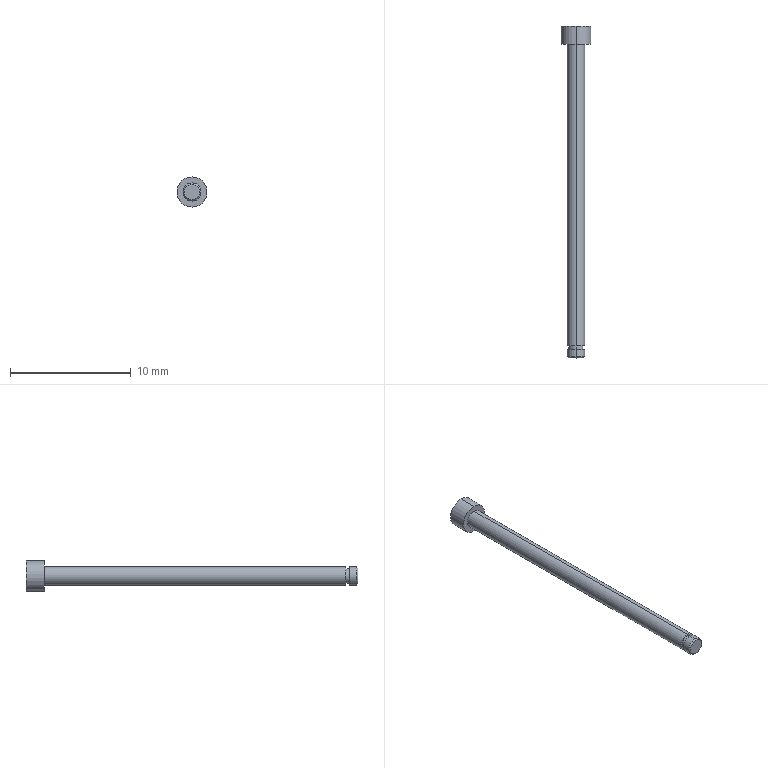Part | SolidWorks | features ICE 2, Chamfer 1, Extrusion 1 | 1 solid | 15 faces | box 2.5 x 27.5 x 2.5 mm | volume 53.096 mm3 | cylinder 8 | plane 5 | cone 2 | commonest cylinder face diameters 1.5 x4 1.2 x2 2.5 x2
STEP:
#1=CARTESIAN_POINT('',(0.,0.,-0.65));
#2=VERTEX_POINT('',#1);
#3=CARTESIAN_POINT('',(0.,0.,0.65));
#4=VERTEX_POINT('',#3);
#5=CARTESIAN_POINT('',(0.,0.,0.));
#6=DIRECTION('',(0.,-1.,0.));
#7=DIRECTION('',(0.,0.,1.));
#8=AXIS2_PLACEMENT_3D('',#5,#6,#7);
#9=CIRCLE('',#8,0.65);
#10=EDGE_CURVE('',#2,#4,#9,.T.);
#11=ORIENTED_EDGE('',*,*,#10,.F.);
#12=CARTESIAN_POINT('',(0.,0.1,-0.75));
#13=VERTEX_POINT('',#12);
#14=CARTESIAN_POINT('',(0.,0.1,-0.75));
#15=DIRECTION('',(0.,0.7071,-0.7071));
#16=VECTOR('',#15,1000.);
#17=LINE('',#14,#16);
#18=EDGE_CURVE('',#2,#13,#17,.T.);
#19=ORIENTED_EDGE('',*,*,#18,.T.);
#20=CARTESIAN_POINT('',(0.,0.1,0.75));
#21=VERTEX_POINT('',#20);
#22=CARTESIAN_POINT('',(0.,0.1,0.));
#23=DIRECTION('',(0.,1.,0.));
#24=DIRECTION('',(0.,0.,1.));
#25=AXIS2_PLACEMENT_3D('',#22,#23,#24);
#26=CIRCLE('',#25,0.75);
#27=EDGE_CURVE('',#21,#13,#26,.T.);
#28=ORIENTED_EDGE('',*,*,#27,.F.);
#29=CARTESIAN_POINT('',(0.,0.1,0.75));
#30=DIRECTION('',(0.,0.7071,0.7071));
#31=VECTOR('',#30,1000.);
#32=LINE('',#29,#31);
#33=EDGE_CURVE('',#4,#21,#32,.T.);
#34=ORIENTED_EDGE('',*,*,#33,.F.);
#35=EDGE_LOOP('',(#11,#19,#28,#34));
#36=FACE_OUTER_BOUND('',#35,.T.);
#37=CARTESIAN_POINT('',(0.,0.1,0.));
#38=DIRECTION('',(0.,1.,0.));
#39=DIRECTION('',(0.,0.,1.));
#40=AXIS2_PLACEMENT_3D('',#37,#38,#39);
#41=CONICAL_SURFACE('',#40,0.75,0.7854);
#42=ADVANCED_FACE('',(#36),#41,.T.);
#43=CARTESIAN_POINT('',(0.,0.7,-0.75));
#44=VERTEX_POINT('',#43);
#45=CARTESIAN_POINT('',(0.,0.7,0.75));
#46=VERTEX_POINT('',#45);
#47=CARTESIAN_POINT('',(0.,0.7,0.));
#48=DIRECTION('',(0.,-1.,0.));
#49=DIRECTION('',(0.,0.,-1.));
#50=AXIS2_PLACEMENT_3D('',#47,#48,#49);
#51=CIRCLE('',#50,0.75);
#52=EDGE_CURVE('',#44,#46,#51,.T.);
#53=ORIENTED_EDGE('',*,*,#52,.T.);
#54=CARTESIAN_POINT('',(0.,26.,0.75));
#55=DIRECTION('',(0.,-1.,0.));
#56=VECTOR('',#55,1000.);
#57=LINE('',#54,#56);
#58=EDGE_CURVE('',#46,#21,#57,.T.);
#59=ORIENTED_EDGE('',*,*,#58,.T.);
#60=ORIENTED_EDGE('',*,*,#27,.T.);
#61=CARTESIAN_POINT('',(0.,26.,-0.75));
#62=DIRECTION('',(0.,-1.,0.));
#63=VECTOR('',#62,1000.);
#64=LINE('',#61,#63);
#65=EDGE_CURVE('',#44,#13,#64,.T.);
#66=ORIENTED_EDGE('',*,*,#65,.F.);
#67=EDGE_LOOP('',(#53,#59,#60,#66));
#68=FACE_OUTER_BOUND('',#67,.T.);
#69=CARTESIAN_POINT('',(0.,26.,0.));
#70=DIRECTION('',(0.,-1.,0.));
#71=DIRECTION('',(0.,0.,-1.));
#72=AXIS2_PLACEMENT_3D('',#69,#70,#71);
#73=CYLINDRICAL_SURFACE('',#72,0.75);
#74=ADVANCED_FACE('',(#68),#73,.T.);
#75=CARTESIAN_POINT('',(0.,0.7,-0.6));
#76=VERTEX_POINT('',#75);
#77=CARTESIAN_POINT('',(0.,0.7,0.6));
#78=VERTEX_POINT('',#77);
#79=CARTESIAN_POINT('',(0.,0.7,0.));
#80=DIRECTION('',(0.,-1.,0.));
#81=DIRECTION('',(0.,0.,-1.));
#82=AXIS2_PLACEMENT_3D('',#79,#80,#81);
#83=CIRCLE('',#82,0.6);
#84=EDGE_CURVE('',#76,#78,#83,.T.);
#85=ORIENTED_EDGE('',*,*,#84,.F.);
#86=CARTESIAN_POINT('',(0.,1.,-0.6));
#87=VERTEX_POINT('',#86);
#88=CARTESIAN_POINT('',(0.,0.7,-0.6));
#89=DIRECTION('',(0.,1.,0.));
#90=VECTOR('',#89,1000.);
#91=LINE('',#88,#90);
#92=EDGE_CURVE('',#76,#87,#91,.T.);
#93=ORIENTED_EDGE('',*,*,#92,.T.);
#94=CARTESIAN_POINT('',(0.,1.,0.6));
#95=VERTEX_POINT('',#94);
#96=CARTESIAN_POINT('',(0.,1.,0.));
#97=DIRECTION('',(0.,-1.,0.));
#98=DIRECTION('',(0.,0.,-1.));
#99=AXIS2_PLACEMENT_3D('',#96,#97,#98);
#100=CIRCLE('',#99,0.6);
#101=EDGE_CURVE('',#87,#95,#100,.T.);
#102=ORIENTED_EDGE('',*,*,#101,.T.);
#103=CARTESIAN_POINT('',(0.,0.7,0.6));
#104=DIRECTION('',(0.,1.,0.));
#105=VECTOR('',#104,1000.);
#106=LINE('',#103,#105);
#107=EDGE_CURVE('',#78,#95,#106,.T.);
#108=ORIENTED_EDGE('',*,*,#107,.F.);
#109=EDGE_LOOP('',(#85,#93,#102,#108));
#110=FACE_OUTER_BOUND('',#109,.T.);
#111=CARTESIAN_POINT('',(0.,0.7,0.));
#112=DIRECTION('',(0.,1.,0.));
#113=DIRECTION('',(0.,0.,1.));
#114=AXIS2_PLACEMENT_3D('',#111,#112,#113);
#115=CYLINDRICAL_SURFACE('',#114,0.6);
#116=ADVANCED_FACE('',(#110),#115,.T.);
#117=CARTESIAN_POINT('',(0.,27.5,1.25));
#118=VERTEX_POINT('',#117);
#119=CARTESIAN_POINT('',(0.,27.5,-1.25));
#120=VERTEX_POINT('',#119);
#121=CARTESIAN_POINT('',(0.,27.5,0.));
#122=DIRECTION('',(0.,1.,0.));
#123=DIRECTION('',(0.,0.,1.));
#124=AXIS2_PLACEMENT_3D('',#121,#122,#123);
#125=CIRCLE('',#124,1.25);
#126=EDGE_CURVE('',#118,#120,#125,.T.);
#127=ORIENTED_EDGE('',*,*,#126,.F.);
#128=CARTESIAN_POINT('',(0.,26.,1.25));
#129=VERTEX_POINT('',#128);
#130=CARTESIAN_POINT('',(0.,27.5,1.25));
#131=DIRECTION('',(0.,-1.,0.));
#132=VECTOR('',#131,1000.);
#133=LINE('',#130,#132);
#134=EDGE_CURVE('',#118,#129,#133,.T.);
#135=ORIENTED_EDGE('',*,*,#134,.T.);
#136=CARTESIAN_POINT('',(0.,26.,-1.25));
#137=VERTEX_POINT('',#136);
#138=CARTESIAN_POINT('',(0.,26.,0.));
#139=DIRECTION('',(0.,1.,0.));
#140=DIRECTION('',(0.,0.,1.));
#141=AXIS2_PLACEMENT_3D('',#138,#139,#140);
#142=CIRCLE('',#141,1.25);
#143=EDGE_CURVE('',#129,#137,#142,.T.);
#144=ORIENTED_EDGE('',*,*,#143,.T.);
#145=CARTESIAN_POINT('',(0.,27.5,-1.25));
#146=DIRECTION('',(0.,-1.,0.));
#147=VECTOR('',#146,1000.);
#148=LINE('',#145,#147);
#149=EDGE_CURVE('',#120,#137,#148,.T.);
#150=ORIENTED_EDGE('',*,*,#149,.F.);
#151=EDGE_LOOP('',(#127,#135,#144,#150));
#152=FACE_OUTER_BOUND('',#151,.T.);
#153=CARTESIAN_POINT('',(0.,27.5,0.));
#154=DIRECTION('',(0.,-1.,0.));
#155=DIRECTION('',(0.,0.,-1.));
#156=AXIS2_PLACEMENT_3D('',#153,#154,#155);
#157=CYLINDRICAL_SURFACE('',#156,1.25);
#158=ADVANCED_FACE('',(#152),#157,.T.);
#159=CARTESIAN_POINT('',(0.,26.,0.75));
#160=VERTEX_POINT('',#159);
#161=CARTESIAN_POINT('',(0.,26.,-0.75));
#162=VERTEX_POINT('',#161);
#163=CARTESIAN_POINT('',(0.,26.,0.));
#164=DIRECTION('',(0.,1.,0.));
#165=DIRECTION('',(0.,0.,1.));
#166=AXIS2_PLACEMENT_3D('',#163,#164,#165);
#167=CIRCLE('',#166,0.75);
#168=EDGE_CURVE('',#160,#162,#167,.T.);
#169=ORIENTED_EDGE('',*,*,#168,.F.);
#170=CARTESIAN_POINT('',(0.,1.,0.75));
#171=VERTEX_POINT('',#170);
#172=CARTESIAN_POINT('',(0.,26.,0.75));
#173=DIRECTION('',(0.,-1.,0.));
#174=VECTOR('',#173,1000.);
#175=LINE('',#172,#174);
#176=EDGE_CURVE('',#160,#171,#175,.T.);
#177=ORIENTED_EDGE('',*,*,#176,.T.);
#178=CARTESIAN_POINT('',(0.,1.,-0.75));
#179=VERTEX_POINT('',#178);
#180=CARTESIAN_POINT('',(0.,1.,0.));
#181=DIRECTION('',(0.,-1.,0.));
#182=DIRECTION('',(0.,0.,-1.));
#183=AXIS2_PLACEMENT_3D('',#180,#181,#182);
#184=CIRCLE('',#183,0.75);
#185=EDGE_CURVE('',#179,#171,#184,.T.);
#186=ORIENTED_EDGE('',*,*,#185,.F.);
#187=CARTESIAN_POINT('',(0.,26.,-0.75));
#188=DIRECTION('',(0.,-1.,0.));
#189=VECTOR('',#188,1000.);
#190=LINE('',#187,#189);
#191=EDGE_CURVE('',#162,#179,#190,.T.);
#192=ORIENTED_EDGE('',*,*,#191,.F.);
#193=EDGE_LOOP('',(#169,#177,#186,#192));
#194=FACE_OUTER_BOUND('',#193,.T.);
#195=CARTESIAN_POINT('',(0.,26.,0.));
#196=DIRECTION('',(0.,-1.,0.));
#197=DIRECTION('',(0.,0.,-1.));
#198=AXIS2_PLACEMENT_3D('',#195,#196,#197);
#199=CYLINDRICAL_SURFACE('',#198,0.75);
#200=ADVANCED_FACE('',(#194),#199,.T.);
#201=ORIENTED_EDGE('',*,*,#176,.F.);
#202=CARTESIAN_POINT('',(0.,26.,0.));
#203=DIRECTION('',(0.,1.,0.));
#204=DIRECTION('',(0.,0.,1.));
#205=AXIS2_PLACEMENT_3D('',#202,#203,#204);
#206=CIRCLE('',#205,0.75);
#207=EDGE_CURVE('',#162,#160,#206,.T.);
#208=ORIENTED_EDGE('',*,*,#207,.F.);
#209=ORIENTED_EDGE('',*,*,#191,.T.);
#210=CARTESIAN_POINT('',(0.,1.,0.));
#211=DIRECTION('',(0.,-1.,0.));
#212=DIRECTION('',(0.,0.,-1.));
#213=AXIS2_PLACEMENT_3D('',#210,#211,#212);
#214=CIRCLE('',#213,0.75);
#215=EDGE_CURVE('',#171,#179,#214,.T.);
#216=ORIENTED_EDGE('',*,*,#215,.F.);
#217=EDGE_LOOP('',(#201,#208,#209,#216));
#218=FACE_OUTER_BOUND('',#217,.T.);
#219=CARTESIAN_POINT('',(0.,26.,0.));
#220=DIRECTION('',(0.,-1.,0.));
#221=DIRECTION('',(0.,0.,-1.));
#222=AXIS2_PLACEMENT_3D('',#219,#220,#221);
#223=CYLINDRICAL_SURFACE('',#222,0.75);
#224=ADVANCED_FACE('',(#218),#223,.T.);
#225=ORIENTED_EDGE('',*,*,#134,.F.);
#226=CARTESIAN_POINT('',(0.,27.5,0.));
#227=DIRECTION('',(0.,1.,0.));
#228=DIRECTION('',(0.,0.,1.));
#229=AXIS2_PLACEMENT_3D('',#226,#227,#228);
#230=CIRCLE('',#229,1.25);
#231=EDGE_CURVE('',#120,#118,#230,.T.);
#232=ORIENTED_EDGE('',*,*,#231,.F.);
#233=ORIENTED_EDGE('',*,*,#149,.T.);
#234=CARTESIAN_POINT('',(0.,26.,0.));
#235=DIRECTION('',(0.,1.,0.));
#236=DIRECTION('',(0.,0.,1.));
#237=AXIS2_PLACEMENT_3D('',#234,#235,#236);
#238=CIRCLE('',#237,1.25);
#239=EDGE_CURVE('',#137,#129,#238,.T.);
#240=ORIENTED_EDGE('',*,*,#239,.T.);
#241=EDGE_LOOP('',(#225,#232,#233,#240));
#242=FACE_OUTER_BOUND('',#241,.T.);
#243=CARTESIAN_POINT('',(0.,27.5,0.));
#244=DIRECTION('',(0.,-1.,0.));
#245=DIRECTION('',(0.,0.,-1.));
#246=AXIS2_PLACEMENT_3D('',#243,#244,#245);
#247=CYLINDRICAL_SURFACE('',#246,1.25);
#248=ADVANCED_FACE('',(#242),#247,.T.);
#249=ORIENTED_EDGE('',*,*,#231,.T.);
#250=ORIENTED_EDGE('',*,*,#126,.T.);
#251=EDGE_LOOP('',(#249,#250));
#252=FACE_OUTER_BOUND('',#251,.T.);
#253=CARTESIAN_POINT('',(0.,27.5,0.));
#254=DIRECTION('',(0.,1.,0.));
#255=DIRECTION('',(0.,0.,1.));
#256=AXIS2_PLACEMENT_3D('',#253,#254,#255);
#257=PLANE('',#256);
#258=ADVANCED_FACE('',(#252),#257,.T.);
#259=ORIENTED_EDGE('',*,*,#207,.T.);
#260=ORIENTED_EDGE('',*,*,#168,.T.);
#261=EDGE_LOOP('',(#259,#260));
#262=FACE_BOUND('',#261,.T.);
#263=ORIENTED_EDGE('',*,*,#239,.F.);
#264=ORIENTED_EDGE('',*,*,#143,.F.);
#265=EDGE_LOOP('',(#263,#264));
#266=FACE_OUTER_BOUND('',#265,.T.);
#267=CARTESIAN_POINT('',(0.,26.,0.));
#268=DIRECTION('',(0.,1.,0.));
#269=DIRECTION('',(0.,0.,1.));
#270=AXIS2_PLACEMENT_3D('',#267,#268,#269);
#271=PLANE('',#270);
#272=ADVANCED_FACE('',(#262,#266),#271,.F.);
#273=CARTESIAN_POINT('',(0.,0.7,0.));
#274=DIRECTION('',(0.,-1.,0.));
#275=DIRECTION('',(0.,0.,-1.));
#276=AXIS2_PLACEMENT_3D('',#273,#274,#275);
#277=CIRCLE('',#276,0.6);
#278=EDGE_CURVE('',#78,#76,#277,.T.);
#279=ORIENTED_EDGE('',*,*,#278,.T.);
#280=ORIENTED_EDGE('',*,*,#84,.T.);
#281=EDGE_LOOP('',(#279,#280));
#282=FACE_BOUND('',#281,.T.);
#283=ORIENTED_EDGE('',*,*,#52,.F.);
#284=CARTESIAN_POINT('',(0.,0.7,0.));
#285=DIRECTION('',(0.,-1.,0.));
#286=DIRECTION('',(0.,0.,-1.));
#287=AXIS2_PLACEMENT_3D('',#284,#285,#286);
#288=CIRCLE('',#287,0.75);
#289=EDGE_CURVE('',#46,#44,#288,.T.);
#290=ORIENTED_EDGE('',*,*,#289,.F.);
#291=EDGE_LOOP('',(#283,#290));
#292=FACE_OUTER_BOUND('',#291,.T.);
#293=CARTESIAN_POINT('',(0.,0.7,0.));
#294=DIRECTION('',(0.,-1.,0.));
#295=DIRECTION('',(0.,0.,-1.));
#296=AXIS2_PLACEMENT_3D('',#293,#294,#295);
#297=PLANE('',#296);
#298=ADVANCED_FACE('',(#282,#292),#297,.F.);
#299=CARTESIAN_POINT('',(0.,1.,0.));
#300=DIRECTION('',(0.,-1.,0.));
#301=DIRECTION('',(0.,0.,-1.));
#302=AXIS2_PLACEMENT_3D('',#299,#300,#301);
#303=CIRCLE('',#302,0.6);
#304=EDGE_CURVE('',#95,#87,#303,.T.);
#305=ORIENTED_EDGE('',*,*,#304,.F.);
#306=ORIENTED_EDGE('',*,*,#101,.F.);
#307=EDGE_LOOP('',(#305,#306));
#308=FACE_BOUND('',#307,.T.);
#309=ORIENTED_EDGE('',*,*,#185,.T.);
#310=ORIENTED_EDGE('',*,*,#215,.T.);
#311=EDGE_LOOP('',(#309,#310));
#312=FACE_OUTER_BOUND('',#311,.T.);
#313=CARTESIAN_POINT('',(0.,1.,0.));
#314=DIRECTION('',(0.,-1.,0.));
#315=DIRECTION('',(0.,0.,-1.));
#316=AXIS2_PLACEMENT_3D('',#313,#314,#315);
#317=PLANE('',#316);
#318=ADVANCED_FACE('',(#308,#312),#317,.T.);
#319=ORIENTED_EDGE('',*,*,#92,.F.);
#320=ORIENTED_EDGE('',*,*,#278,.F.);
#321=ORIENTED_EDGE('',*,*,#107,.T.);
#322=ORIENTED_EDGE('',*,*,#304,.T.);
#323=EDGE_LOOP('',(#319,#320,#321,#322));
#324=FACE_OUTER_BOUND('',#323,.T.);
#325=CARTESIAN_POINT('',(0.,0.7,0.));
#326=DIRECTION('',(0.,1.,0.));
#327=DIRECTION('',(0.,0.,1.));
#328=AXIS2_PLACEMENT_3D('',#325,#326,#327);
#329=CYLINDRICAL_SURFACE('',#328,0.6);
#330=ADVANCED_FACE('',(#324),#329,.T.);
#331=CARTESIAN_POINT('',(0.,0.,0.));
#332=DIRECTION('',(0.,-1.,0.));
#333=DIRECTION('',(0.,0.,1.));
#334=AXIS2_PLACEMENT_3D('',#331,#332,#333);
#335=CIRCLE('',#334,0.65);
#336=EDGE_CURVE('',#4,#2,#335,.T.);
#337=ORIENTED_EDGE('',*,*,#336,.T.);
#338=ORIENTED_EDGE('',*,*,#10,.T.);
#339=EDGE_LOOP('',(#337,#338));
#340=FACE_OUTER_BOUND('',#339,.T.);
#341=CARTESIAN_POINT('',(0.,0.,0.));
#342=DIRECTION('',(0.,1.,0.));
#343=DIRECTION('',(0.,0.,1.));
#344=AXIS2_PLACEMENT_3D('',#341,#342,#343);
#345=PLANE('',#344);
#346=ADVANCED_FACE('',(#340),#345,.F.);
#347=ORIENTED_EDGE('',*,*,#58,.F.);
#348=ORIENTED_EDGE('',*,*,#289,.T.);
#349=ORIENTED_EDGE('',*,*,#65,.T.);
#350=CARTESIAN_POINT('',(0.,0.1,0.));
#351=DIRECTION('',(0.,1.,0.));
#352=DIRECTION('',(0.,0.,1.));
#353=AXIS2_PLACEMENT_3D('',#350,#351,#352);
#354=CIRCLE('',#353,0.75);
#355=EDGE_CURVE('',#13,#21,#354,.T.);
#356=ORIENTED_EDGE('',*,*,#355,.T.);
#357=EDGE_LOOP('',(#347,#348,#349,#356));
#358=FACE_OUTER_BOUND('',#357,.T.);
#359=CARTESIAN_POINT('',(0.,26.,0.));
#360=DIRECTION('',(0.,-1.,0.));
#361=DIRECTION('',(0.,0.,-1.));
#362=AXIS2_PLACEMENT_3D('',#359,#360,#361);
#363=CYLINDRICAL_SURFACE('',#362,0.75);
#364=ADVANCED_FACE('',(#358),#363,.T.);
#365=ORIENTED_EDGE('',*,*,#18,.F.);
#366=ORIENTED_EDGE('',*,*,#336,.F.);
#367=ORIENTED_EDGE('',*,*,#33,.T.);
#368=ORIENTED_EDGE('',*,*,#355,.F.);
#369=EDGE_LOOP('',(#365,#366,#367,#368));
#370=FACE_OUTER_BOUND('',#369,.T.);
#371=CARTESIAN_POINT('',(0.,0.1,0.));
#372=DIRECTION('',(0.,1.,0.));
#373=DIRECTION('',(0.,0.,1.));
#374=AXIS2_PLACEMENT_3D('',#371,#372,#373);
#375=CONICAL_SURFACE('',#374,0.75,0.7854);
#376=ADVANCED_FACE('',(#370),#375,.T.);
#377=CLOSED_SHELL('',(#42,#74,#116,#158,#200,#224,#248,#258,#272,#298,#318,#330,#346,#364,#376));
#378=MANIFOLD_SOLID_BREP('',#377);
#379=CARTESIAN_POINT('',(0.,0.,0.));
#380=DIRECTION('',(0.,0.,1.));
#381=DIRECTION('',(1.,0.,0.));
#382=AXIS2_PLACEMENT_3D('',#379,#380,#381);
#383=(LENGTH_UNIT()NAMED_UNIT(*)SI_UNIT(.MILLI.,.METRE.));
#384=UNCERTAINTY_MEASURE_WITH_UNIT(LENGTH_MEASURE(0.00001),#383,'','');
#385=(NAMED_UNIT(*)PLANE_ANGLE_UNIT()SI_UNIT($,.RADIAN.));
#386=(NAMED_UNIT(*)SI_UNIT($,.STERADIAN.)SOLID_ANGLE_UNIT());
#387=(GEOMETRIC_REPRESENTATION_CONTEXT(3)GLOBAL_UNCERTAINTY_ASSIGNED_CONTEXT((#384))GLOBAL_UNIT_ASSIGNED_CONTEXT((#383,#385,#386))REPRESENTATION_CONTEXT('',''));
#388=ADVANCED_BREP_SHAPE_REPRESENTATION('',(#378,#382),#387);